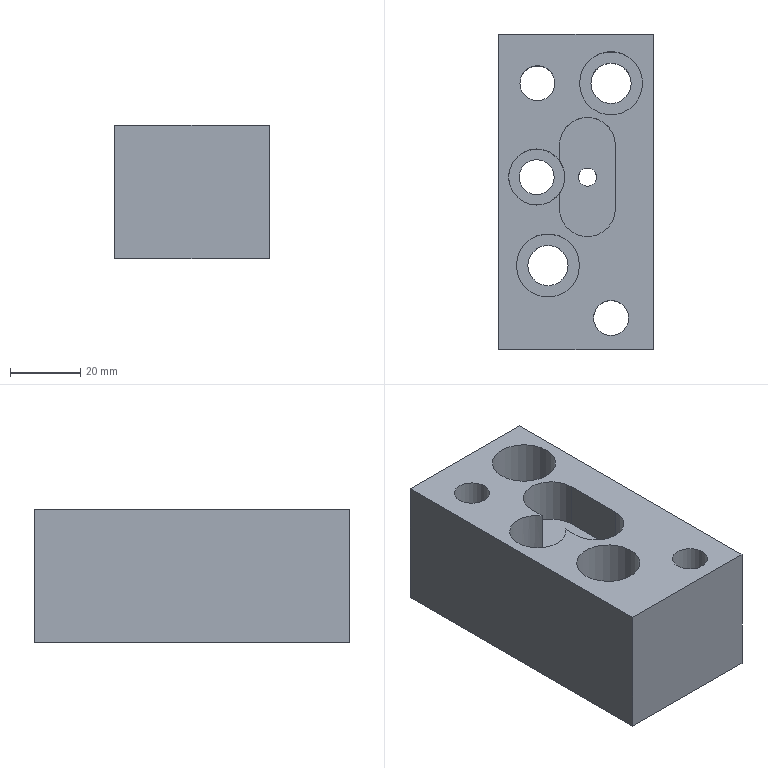Part | STEP file | lll_id142_x_t | 1 solid | 24 faces | box 44 x 90 x 38 mm | volume 119506 mm3 | plane 13 | cylinder 11 | commonest cylinder face diameters 10 x3 16 x3 11.509 x2 18.008 x2 5.206 x1
STEP:
#1=CARTESIAN_POINT('',(784.996,-55.25,0.));
#2=VERTEX_POINT('',#1);
#3=CARTESIAN_POINT('',(794.,-55.25,0.));
#4=DIRECTION('',(0.,0.,-1.));
#5=DIRECTION('',(-1.,0.,0.));
#6=AXIS2_PLACEMENT_3D('',#3,#4,#5);
#7=CIRCLE('',#6,9.004);
#8=EDGE_CURVE('',#2,#2,#7,.T.);
#9=ORIENTED_EDGE('',*,*,#8,.T.);
#10=EDGE_LOOP('',(#9));
#11=FACE_BOUND('',#10,.T.);
#12=CARTESIAN_POINT('',(780.,-79.25,0.));
#13=VERTEX_POINT('',#12);
#14=CARTESIAN_POINT('',(780.,10.75,0.));
#15=VERTEX_POINT('',#14);
#16=CARTESIAN_POINT('',(780.,0.,0.));
#17=DIRECTION('',(0.,1.,0.));
#18=VECTOR('',#17,1.);
#19=LINE('',#16,#18);
#20=EDGE_CURVE('',#13,#15,#19,.T.);
#21=ORIENTED_EDGE('',*,*,#20,.F.);
#22=CARTESIAN_POINT('',(824.,-79.25,0.));
#23=VERTEX_POINT('',#22);
#24=CARTESIAN_POINT('',(829.,-79.25,0.));
#25=DIRECTION('',(-1.,0.,0.));
#26=VECTOR('',#25,1.);
#27=LINE('',#24,#26);
#28=EDGE_CURVE('',#23,#13,#27,.T.);
#29=ORIENTED_EDGE('',*,*,#28,.F.);
#30=CARTESIAN_POINT('',(824.,10.75,0.));
#31=VERTEX_POINT('',#30);
#32=CARTESIAN_POINT('',(824.,0.,0.));
#33=DIRECTION('',(0.,1.,0.));
#34=VECTOR('',#33,1.);
#35=LINE('',#32,#34);
#36=EDGE_CURVE('',#23,#31,#35,.T.);
#37=ORIENTED_EDGE('',*,*,#36,.T.);
#38=CARTESIAN_POINT('',(829.,10.75,0.));
#39=DIRECTION('',(-1.,0.,0.));
#40=VECTOR('',#39,1.);
#41=LINE('',#38,#40);
#42=EDGE_CURVE('',#31,#15,#41,.T.);
#43=ORIENTED_EDGE('',*,*,#42,.T.);
#44=EDGE_LOOP('',(#21,#29,#37,#43));
#45=FACE_BOUND('',#44,.T.);
#46=CARTESIAN_POINT('',(796.,-3.25,0.));
#47=VERTEX_POINT('',#46);
#48=CARTESIAN_POINT('',(791.,-3.25,0.));
#49=DIRECTION('',(0.,0.,1.));
#50=DIRECTION('',(1.,0.,0.));
#51=AXIS2_PLACEMENT_3D('',#48,#49,#50);
#52=CIRCLE('',#51,5.);
#53=EDGE_CURVE('',#47,#47,#52,.T.);
#54=ORIENTED_EDGE('',*,*,#53,.F.);
#55=EDGE_LOOP('',(#54));
#56=FACE_BOUND('',#55,.T.);
#57=CARTESIAN_POINT('',(802.996,-3.25,0.));
#58=VERTEX_POINT('',#57);
#59=CARTESIAN_POINT('',(812.,-3.25,0.));
#60=DIRECTION('',(0.,0.,-1.));
#61=DIRECTION('',(-1.,0.,0.));
#62=AXIS2_PLACEMENT_3D('',#59,#60,#61);
#63=CIRCLE('',#62,9.004);
#64=EDGE_CURVE('',#58,#58,#63,.T.);
#65=ORIENTED_EDGE('',*,*,#64,.T.);
#66=EDGE_LOOP('',(#65));
#67=FACE_BOUND('',#66,.T.);
#68=CARTESIAN_POINT('',(817.,-70.25,0.));
#69=VERTEX_POINT('',#68);
#70=CARTESIAN_POINT('',(812.,-70.25,0.));
#71=DIRECTION('',(0.,0.,1.));
#72=DIRECTION('',(1.,0.,0.));
#73=AXIS2_PLACEMENT_3D('',#70,#71,#72);
#74=CIRCLE('',#73,5.);
#75=EDGE_CURVE('',#69,#69,#74,.T.);
#76=ORIENTED_EDGE('',*,*,#75,.F.);
#77=EDGE_LOOP('',(#76));
#78=FACE_BOUND('',#77,.T.);
#79=CARTESIAN_POINT('',(797.273,-39.,0.));
#80=VERTEX_POINT('',#79);
#81=CARTESIAN_POINT('',(813.273,-39.,0.));
#82=VERTEX_POINT('',#81);
#83=CARTESIAN_POINT('',(805.273,-39.,0.));
#84=DIRECTION('',(0.,0.,1.));
#85=DIRECTION('',(1.,0.,0.));
#86=AXIS2_PLACEMENT_3D('',#83,#84,#85);
#87=CIRCLE('',#86,8.);
#88=EDGE_CURVE('',#80,#82,#87,.T.);
#89=ORIENTED_EDGE('',*,*,#88,.F.);
#90=CARTESIAN_POINT('',(797.273,-34.664,0.));
#91=VERTEX_POINT('',#90);
#92=CARTESIAN_POINT('',(797.273,-79.25,0.));
#93=DIRECTION('',(0.,1.,0.));
#94=VECTOR('',#93,1.);
#95=LINE('',#92,#94);
#96=EDGE_CURVE('',#80,#91,#95,.T.);
#97=ORIENTED_EDGE('',*,*,#96,.T.);
#98=CARTESIAN_POINT('',(797.273,-25.336,0.));
#99=VERTEX_POINT('',#98);
#100=CARTESIAN_POINT('',(790.773,-30.,0.));
#101=DIRECTION('',(0.,0.,1.));
#102=DIRECTION('',(1.,0.,0.));
#103=AXIS2_PLACEMENT_3D('',#100,#101,#102);
#104=CIRCLE('',#103,8.);
#105=EDGE_CURVE('',#99,#91,#104,.T.);
#106=ORIENTED_EDGE('',*,*,#105,.F.);
#107=CARTESIAN_POINT('',(797.273,-21.,0.));
#108=VERTEX_POINT('',#107);
#109=CARTESIAN_POINT('',(797.273,-79.25,0.));
#110=DIRECTION('',(0.,1.,0.));
#111=VECTOR('',#110,1.);
#112=LINE('',#109,#111);
#113=EDGE_CURVE('',#99,#108,#112,.T.);
#114=ORIENTED_EDGE('',*,*,#113,.T.);
#115=CARTESIAN_POINT('',(813.273,-21.,0.));
#116=VERTEX_POINT('',#115);
#117=CARTESIAN_POINT('',(805.273,-21.,0.));
#118=DIRECTION('',(0.,0.,1.));
#119=DIRECTION('',(1.,0.,0.));
#120=AXIS2_PLACEMENT_3D('',#117,#118,#119);
#121=CIRCLE('',#120,8.);
#122=EDGE_CURVE('',#116,#108,#121,.T.);
#123=ORIENTED_EDGE('',*,*,#122,.F.);
#124=CARTESIAN_POINT('',(813.273,-79.25,0.));
#125=DIRECTION('',(0.,1.,0.));
#126=VECTOR('',#125,1.);
#127=LINE('',#124,#126);
#128=EDGE_CURVE('',#82,#116,#127,.T.);
#129=ORIENTED_EDGE('',*,*,#128,.F.);
#130=EDGE_LOOP('',(#89,#97,#106,#114,#123,#129));
#131=FACE_BOUND('',#130,.T.);
#132=CARTESIAN_POINT('',(829.,-79.25,0.));
#133=DIRECTION('',(0.,0.,1.));
#134=DIRECTION('',(1.,0.,0.));
#135=AXIS2_PLACEMENT_3D('',#132,#133,#134);
#136=PLANE('',#135);
#137=ADVANCED_FACE('',(#11,#45,#56,#67,#78,#131),#136,.T.);
#138=CARTESIAN_POINT('',(798.773,-30.,-28.));
#139=VERTEX_POINT('',#138);
#140=CARTESIAN_POINT('',(790.773,-30.,-28.));
#141=DIRECTION('',(0.,0.,-1.));
#142=DIRECTION('',(1.,0.,0.));
#143=AXIS2_PLACEMENT_3D('',#140,#141,#142);
#144=CIRCLE('',#143,8.);
#145=EDGE_CURVE('',#139,#139,#144,.T.);
#146=ORIENTED_EDGE('',*,*,#145,.T.);
#147=EDGE_LOOP('',(#146));
#148=FACE_BOUND('',#147,.T.);
#149=CARTESIAN_POINT('',(797.273,-25.336,-13.));
#150=VERTEX_POINT('',#149);
#151=CARTESIAN_POINT('',(797.273,-25.336,0.));
#152=DIRECTION('',(0.,0.,-1.));
#153=VECTOR('',#152,1.);
#154=LINE('',#151,#153);
#155=EDGE_CURVE('',#99,#150,#154,.T.);
#156=ORIENTED_EDGE('',*,*,#155,.F.);
#157=ORIENTED_EDGE('',*,*,#105,.T.);
#158=CARTESIAN_POINT('',(797.273,-34.664,-13.));
#159=VERTEX_POINT('',#158);
#160=CARTESIAN_POINT('',(797.273,-34.664,-13.));
#161=DIRECTION('',(0.,0.,1.));
#162=VECTOR('',#161,1.);
#163=LINE('',#160,#162);
#164=EDGE_CURVE('',#159,#91,#163,.T.);
#165=ORIENTED_EDGE('',*,*,#164,.F.);
#166=CARTESIAN_POINT('',(790.773,-30.,-13.));
#167=DIRECTION('',(0.,0.,1.));
#168=DIRECTION('',(-1.,0.,0.));
#169=AXIS2_PLACEMENT_3D('',#166,#167,#168);
#170=CIRCLE('',#169,8.);
#171=EDGE_CURVE('',#159,#150,#170,.T.);
#172=ORIENTED_EDGE('',*,*,#171,.T.);
#173=EDGE_LOOP('',(#156,#157,#165,#172));
#174=FACE_BOUND('',#173,.T.);
#175=CARTESIAN_POINT('',(790.773,-30.,-28.));
#176=DIRECTION('',(0.,0.,1.));
#177=DIRECTION('',(1.,0.,0.));
#178=AXIS2_PLACEMENT_3D('',#175,#176,#177);
#179=CYLINDRICAL_SURFACE('',#178,8.);
#180=ADVANCED_FACE('',(#148,#174),#179,.F.);
#181=CARTESIAN_POINT('',(780.,10.75,-38.));
#182=VERTEX_POINT('',#181);
#183=CARTESIAN_POINT('',(780.,10.75,0.));
#184=DIRECTION('',(0.,0.,-1.));
#185=VECTOR('',#184,1.);
#186=LINE('',#183,#185);
#187=EDGE_CURVE('',#15,#182,#186,.T.);
#188=ORIENTED_EDGE('',*,*,#187,.F.);
#189=ORIENTED_EDGE('',*,*,#42,.F.);
#190=CARTESIAN_POINT('',(824.,10.75,-38.));
#191=VERTEX_POINT('',#190);
#192=CARTESIAN_POINT('',(824.,10.75,0.));
#193=DIRECTION('',(0.,0.,-1.));
#194=VECTOR('',#193,1.);
#195=LINE('',#192,#194);
#196=EDGE_CURVE('',#31,#191,#195,.T.);
#197=ORIENTED_EDGE('',*,*,#196,.T.);
#198=CARTESIAN_POINT('',(829.,10.75,-38.));
#199=DIRECTION('',(-1.,0.,0.));
#200=VECTOR('',#199,1.);
#201=LINE('',#198,#200);
#202=EDGE_CURVE('',#191,#182,#201,.T.);
#203=ORIENTED_EDGE('',*,*,#202,.T.);
#204=EDGE_LOOP('',(#188,#189,#197,#203));
#205=FACE_OUTER_BOUND('',#204,.T.);
#206=CARTESIAN_POINT('',(829.,10.75,0.));
#207=DIRECTION('',(0.,1.,0.));
#208=DIRECTION('',(0.,0.,1.));
#209=AXIS2_PLACEMENT_3D('',#206,#207,#208);
#210=PLANE('',#209);
#211=ADVANCED_FACE('',(#205),#210,.T.);
#212=CARTESIAN_POINT('',(802.67,-30.,-38.));
#213=VERTEX_POINT('',#212);
#214=CARTESIAN_POINT('',(805.273,-30.,-38.));
#215=DIRECTION('',(0.,0.,-1.));
#216=DIRECTION('',(-1.,0.,0.));
#217=AXIS2_PLACEMENT_3D('',#214,#215,#216);
#218=CIRCLE('',#217,2.603);
#219=EDGE_CURVE('',#213,#213,#218,.T.);
#220=ORIENTED_EDGE('',*,*,#219,.F.);
#221=EDGE_LOOP('',(#220));
#222=FACE_BOUND('',#221,.T.);
#223=CARTESIAN_POINT('',(785.773,-30.,-38.));
#224=VERTEX_POINT('',#223);
#225=CARTESIAN_POINT('',(790.773,-30.,-38.));
#226=DIRECTION('',(0.,0.,-1.));
#227=DIRECTION('',(-1.,0.,0.));
#228=AXIS2_PLACEMENT_3D('',#225,#226,#227);
#229=CIRCLE('',#228,5.);
#230=EDGE_CURVE('',#224,#224,#229,.T.);
#231=ORIENTED_EDGE('',*,*,#230,.F.);
#232=EDGE_LOOP('',(#231));
#233=FACE_BOUND('',#232,.T.);
#234=CARTESIAN_POINT('',(807.,-70.25,-38.));
#235=VERTEX_POINT('',#234);
#236=CARTESIAN_POINT('',(812.,-70.25,-38.));
#237=DIRECTION('',(0.,0.,-1.));
#238=DIRECTION('',(-1.,0.,0.));
#239=AXIS2_PLACEMENT_3D('',#236,#237,#238);
#240=CIRCLE('',#239,5.);
#241=EDGE_CURVE('',#235,#235,#240,.T.);
#242=ORIENTED_EDGE('',*,*,#241,.F.);
#243=EDGE_LOOP('',(#242));
#244=FACE_BOUND('',#243,.T.);
#245=CARTESIAN_POINT('',(788.245,-55.25,-38.));
#246=VERTEX_POINT('',#245);
#247=CARTESIAN_POINT('',(794.,-55.25,-38.));
#248=DIRECTION('',(0.,0.,-1.));
#249=DIRECTION('',(-1.,0.,0.));
#250=AXIS2_PLACEMENT_3D('',#247,#248,#249);
#251=CIRCLE('',#250,5.755);
#252=EDGE_CURVE('',#246,#246,#251,.T.);
#253=ORIENTED_EDGE('',*,*,#252,.F.);
#254=EDGE_LOOP('',(#253));
#255=FACE_BOUND('',#254,.T.);
#256=CARTESIAN_POINT('',(806.245,-3.25,-38.));
#257=VERTEX_POINT('',#256);
#258=CARTESIAN_POINT('',(812.,-3.25,-38.));
#259=DIRECTION('',(0.,0.,-1.));
#260=DIRECTION('',(-1.,0.,0.));
#261=AXIS2_PLACEMENT_3D('',#258,#259,#260);
#262=CIRCLE('',#261,5.755);
#263=EDGE_CURVE('',#257,#257,#262,.T.);
#264=ORIENTED_EDGE('',*,*,#263,.F.);
#265=EDGE_LOOP('',(#264));
#266=FACE_BOUND('',#265,.T.);
#267=CARTESIAN_POINT('',(786.,-3.25,-38.));
#268=VERTEX_POINT('',#267);
#269=CARTESIAN_POINT('',(791.,-3.25,-38.));
#270=DIRECTION('',(0.,0.,-1.));
#271=DIRECTION('',(-1.,0.,0.));
#272=AXIS2_PLACEMENT_3D('',#269,#270,#271);
#273=CIRCLE('',#272,5.);
#274=EDGE_CURVE('',#268,#268,#273,.T.);
#275=ORIENTED_EDGE('',*,*,#274,.F.);
#276=EDGE_LOOP('',(#275));
#277=FACE_BOUND('',#276,.T.);
#278=CARTESIAN_POINT('',(780.,-79.25,-38.));
#279=VERTEX_POINT('',#278);
#280=CARTESIAN_POINT('',(780.,0.,-38.));
#281=DIRECTION('',(0.,-1.,0.));
#282=VECTOR('',#281,1.);
#283=LINE('',#280,#282);
#284=EDGE_CURVE('',#182,#279,#283,.T.);
#285=ORIENTED_EDGE('',*,*,#284,.F.);
#286=ORIENTED_EDGE('',*,*,#202,.F.);
#287=CARTESIAN_POINT('',(824.,-79.25,-38.));
#288=VERTEX_POINT('',#287);
#289=CARTESIAN_POINT('',(824.,0.,-38.));
#290=DIRECTION('',(0.,-1.,0.));
#291=VECTOR('',#290,1.);
#292=LINE('',#289,#291);
#293=EDGE_CURVE('',#191,#288,#292,.T.);
#294=ORIENTED_EDGE('',*,*,#293,.T.);
#295=CARTESIAN_POINT('',(829.,-79.25,-38.));
#296=DIRECTION('',(-1.,0.,0.));
#297=VECTOR('',#296,1.);
#298=LINE('',#295,#297);
#299=EDGE_CURVE('',#288,#279,#298,.T.);
#300=ORIENTED_EDGE('',*,*,#299,.T.);
#301=EDGE_LOOP('',(#285,#286,#294,#300));
#302=FACE_BOUND('',#301,.T.);
#303=CARTESIAN_POINT('',(829.,-19.25,-38.));
#304=DIRECTION('',(0.,0.,-1.));
#305=DIRECTION('',(-1.,0.,0.));
#306=AXIS2_PLACEMENT_3D('',#303,#304,#305);
#307=PLANE('',#306);
#308=ADVANCED_FACE('',(#222,#233,#244,#255,#266,#277,#302),#307,.T.);
#309=CARTESIAN_POINT('',(780.,-79.25,0.));
#310=DIRECTION('',(0.,0.,1.));
#311=VECTOR('',#310,1.);
#312=LINE('',#309,#311);
#313=EDGE_CURVE('',#279,#13,#312,.T.);
#314=ORIENTED_EDGE('',*,*,#313,.F.);
#315=ORIENTED_EDGE('',*,*,#299,.F.);
#316=CARTESIAN_POINT('',(824.,-79.25,0.));
#317=DIRECTION('',(0.,0.,1.));
#318=VECTOR('',#317,1.);
#319=LINE('',#316,#318);
#320=EDGE_CURVE('',#288,#23,#319,.T.);
#321=ORIENTED_EDGE('',*,*,#320,.T.);
#322=ORIENTED_EDGE('',*,*,#28,.T.);
#323=EDGE_LOOP('',(#314,#315,#321,#322));
#324=FACE_OUTER_BOUND('',#323,.T.);
#325=CARTESIAN_POINT('',(829.,-79.25,-38.));
#326=DIRECTION('',(0.,-1.,0.));
#327=DIRECTION('',(0.,0.,-1.));
#328=AXIS2_PLACEMENT_3D('',#325,#326,#327);
#329=PLANE('',#328);
#330=ADVANCED_FACE('',(#324),#329,.T.);
#331=ORIENTED_EDGE('',*,*,#196,.F.);
#332=ORIENTED_EDGE('',*,*,#36,.F.);
#333=ORIENTED_EDGE('',*,*,#320,.F.);
#334=ORIENTED_EDGE('',*,*,#293,.F.);
#335=EDGE_LOOP('',(#331,#332,#333,#334));
#336=FACE_OUTER_BOUND('',#335,.T.);
#337=CARTESIAN_POINT('',(824.,0.,0.));
#338=DIRECTION('',(-1.,0.,0.));
#339=DIRECTION('',(0.,0.,1.));
#340=AXIS2_PLACEMENT_3D('',#337,#338,#339);
#341=PLANE('',#340);
#342=ADVANCED_FACE('',(#336),#341,.F.);
#343=ORIENTED_EDGE('',*,*,#187,.T.);
#344=ORIENTED_EDGE('',*,*,#284,.T.);
#345=ORIENTED_EDGE('',*,*,#313,.T.);
#346=ORIENTED_EDGE('',*,*,#20,.T.);
#347=EDGE_LOOP('',(#343,#344,#345,#346));
#348=FACE_OUTER_BOUND('',#347,.T.);
#349=CARTESIAN_POINT('',(780.,0.,0.));
#350=DIRECTION('',(-1.,0.,0.));
#351=DIRECTION('',(0.,0.,1.));
#352=AXIS2_PLACEMENT_3D('',#349,#350,#351);
#353=PLANE('',#352);
#354=ADVANCED_FACE('',(#348),#353,.T.);
#355=ORIENTED_EDGE('',*,*,#274,.T.);
#356=EDGE_LOOP('',(#355));
#357=FACE_BOUND('',#356,.T.);
#358=ORIENTED_EDGE('',*,*,#53,.T.);
#359=EDGE_LOOP('',(#358));
#360=FACE_BOUND('',#359,.T.);
#361=CARTESIAN_POINT('',(791.,-3.25,2.));
#362=DIRECTION('',(0.,0.,-1.));
#363=DIRECTION('',(-1.,0.,0.));
#364=AXIS2_PLACEMENT_3D('',#361,#362,#363);
#365=CYLINDRICAL_SURFACE('',#364,5.);
#366=ADVANCED_FACE('',(#357,#360),#365,.F.);
#367=ORIENTED_EDGE('',*,*,#263,.T.);
#368=EDGE_LOOP('',(#367));
#369=FACE_BOUND('',#368,.T.);
#370=CARTESIAN_POINT('',(806.245,-3.25,-13.));
#371=VERTEX_POINT('',#370);
#372=CARTESIAN_POINT('',(812.,-3.25,-13.));
#373=DIRECTION('',(0.,0.,-1.));
#374=DIRECTION('',(-1.,0.,0.));
#375=AXIS2_PLACEMENT_3D('',#372,#373,#374);
#376=CIRCLE('',#375,5.755);
#377=EDGE_CURVE('',#371,#371,#376,.T.);
#378=ORIENTED_EDGE('',*,*,#377,.F.);
#379=EDGE_LOOP('',(#378));
#380=FACE_BOUND('',#379,.T.);
#381=CARTESIAN_POINT('',(812.,-3.25,2.));
#382=DIRECTION('',(0.,0.,-1.));
#383=DIRECTION('',(-1.,0.,0.));
#384=AXIS2_PLACEMENT_3D('',#381,#382,#383);
#385=CYLINDRICAL_SURFACE('',#384,5.755);
#386=ADVANCED_FACE('',(#369,#380),#385,.F.);
#387=ORIENTED_EDGE('',*,*,#377,.T.);
#388=EDGE_LOOP('',(#387));
#389=FACE_BOUND('',#388,.T.);
#390=CARTESIAN_POINT('',(802.996,-3.25,-13.));
#391=VERTEX_POINT('',#390);
#392=CARTESIAN_POINT('',(812.,-3.25,-13.));
#393=DIRECTION('',(0.,0.,-1.));
#394=DIRECTION('',(-1.,0.,0.));
#395=AXIS2_PLACEMENT_3D('',#392,#393,#394);
#396=CIRCLE('',#395,9.004);
#397=EDGE_CURVE('',#391,#391,#396,.T.);
#398=ORIENTED_EDGE('',*,*,#397,.F.);
#399=EDGE_LOOP('',(#398));
#400=FACE_BOUND('',#399,.T.);
#401=CARTESIAN_POINT('',(812.,-3.25,-13.));
#402=DIRECTION('',(0.,0.,-1.));
#403=DIRECTION('',(-1.,0.,0.));
#404=AXIS2_PLACEMENT_3D('',#401,#402,#403);
#405=PLANE('',#404);
#406=ADVANCED_FACE('',(#389,#400),#405,.F.);
#407=ORIENTED_EDGE('',*,*,#397,.T.);
#408=EDGE_LOOP('',(#407));
#409=FACE_BOUND('',#408,.T.);
#410=ORIENTED_EDGE('',*,*,#64,.F.);
#411=EDGE_LOOP('',(#410));
#412=FACE_BOUND('',#411,.T.);
#413=CARTESIAN_POINT('',(812.,-3.25,0.));
#414=DIRECTION('',(0.,0.,-1.));
#415=DIRECTION('',(-1.,0.,0.));
#416=AXIS2_PLACEMENT_3D('',#413,#414,#415);
#417=CYLINDRICAL_SURFACE('',#416,9.004);
#418=ADVANCED_FACE('',(#409,#412),#417,.F.);
#419=ORIENTED_EDGE('',*,*,#252,.T.);
#420=EDGE_LOOP('',(#419));
#421=FACE_BOUND('',#420,.T.);
#422=CARTESIAN_POINT('',(788.245,-55.25,-13.));
#423=VERTEX_POINT('',#422);
#424=CARTESIAN_POINT('',(794.,-55.25,-13.));
#425=DIRECTION('',(0.,0.,-1.));
#426=DIRECTION('',(-1.,0.,0.));
#427=AXIS2_PLACEMENT_3D('',#424,#425,#426);
#428=CIRCLE('',#427,5.755);
#429=EDGE_CURVE('',#423,#423,#428,.T.);
#430=ORIENTED_EDGE('',*,*,#429,.F.);
#431=EDGE_LOOP('',(#430));
#432=FACE_BOUND('',#431,.T.);
#433=CARTESIAN_POINT('',(794.,-55.25,2.));
#434=DIRECTION('',(0.,0.,-1.));
#435=DIRECTION('',(-1.,0.,0.));
#436=AXIS2_PLACEMENT_3D('',#433,#434,#435);
#437=CYLINDRICAL_SURFACE('',#436,5.755);
#438=ADVANCED_FACE('',(#421,#432),#437,.F.);
#439=ORIENTED_EDGE('',*,*,#429,.T.);
#440=EDGE_LOOP('',(#439));
#441=FACE_BOUND('',#440,.T.);
#442=CARTESIAN_POINT('',(784.996,-55.25,-13.));
#443=VERTEX_POINT('',#442);
#444=CARTESIAN_POINT('',(794.,-55.25,-13.));
#445=DIRECTION('',(0.,0.,-1.));
#446=DIRECTION('',(-1.,0.,0.));
#447=AXIS2_PLACEMENT_3D('',#444,#445,#446);
#448=CIRCLE('',#447,9.004);
#449=EDGE_CURVE('',#443,#443,#448,.T.);
#450=ORIENTED_EDGE('',*,*,#449,.F.);
#451=EDGE_LOOP('',(#450));
#452=FACE_BOUND('',#451,.T.);
#453=CARTESIAN_POINT('',(794.,-55.25,-13.));
#454=DIRECTION('',(0.,0.,-1.));
#455=DIRECTION('',(-1.,0.,0.));
#456=AXIS2_PLACEMENT_3D('',#453,#454,#455);
#457=PLANE('',#456);
#458=ADVANCED_FACE('',(#441,#452),#457,.F.);
#459=ORIENTED_EDGE('',*,*,#449,.T.);
#460=EDGE_LOOP('',(#459));
#461=FACE_BOUND('',#460,.T.);
#462=ORIENTED_EDGE('',*,*,#8,.F.);
#463=EDGE_LOOP('',(#462));
#464=FACE_BOUND('',#463,.T.);
#465=CARTESIAN_POINT('',(794.,-55.25,0.));
#466=DIRECTION('',(0.,0.,-1.));
#467=DIRECTION('',(-1.,0.,0.));
#468=AXIS2_PLACEMENT_3D('',#465,#466,#467);
#469=CYLINDRICAL_SURFACE('',#468,9.004);
#470=ADVANCED_FACE('',(#461,#464),#469,.F.);
#471=ORIENTED_EDGE('',*,*,#75,.T.);
#472=EDGE_LOOP('',(#471));
#473=FACE_BOUND('',#472,.T.);
#474=ORIENTED_EDGE('',*,*,#241,.T.);
#475=EDGE_LOOP('',(#474));
#476=FACE_BOUND('',#475,.T.);
#477=CARTESIAN_POINT('',(812.,-70.25,2.));
#478=DIRECTION('',(0.,0.,-1.));
#479=DIRECTION('',(-1.,0.,0.));
#480=AXIS2_PLACEMENT_3D('',#477,#478,#479);
#481=CYLINDRICAL_SURFACE('',#480,5.);
#482=ADVANCED_FACE('',(#473,#476),#481,.F.);
#483=CARTESIAN_POINT('',(785.773,-30.,-28.));
#484=VERTEX_POINT('',#483);
#485=CARTESIAN_POINT('',(790.773,-30.,-28.));
#486=DIRECTION('',(0.,0.,-1.));
#487=DIRECTION('',(-1.,0.,0.));
#488=AXIS2_PLACEMENT_3D('',#485,#486,#487);
#489=CIRCLE('',#488,5.);
#490=EDGE_CURVE('',#484,#484,#489,.T.);
#491=ORIENTED_EDGE('',*,*,#490,.T.);
#492=EDGE_LOOP('',(#491));
#493=FACE_BOUND('',#492,.T.);
#494=ORIENTED_EDGE('',*,*,#145,.F.);
#495=EDGE_LOOP('',(#494));
#496=FACE_BOUND('',#495,.T.);
#497=CARTESIAN_POINT('',(790.773,-30.,-28.));
#498=DIRECTION('',(0.,0.,-1.));
#499=DIRECTION('',(-1.,0.,0.));
#500=AXIS2_PLACEMENT_3D('',#497,#498,#499);
#501=PLANE('',#500);
#502=ADVANCED_FACE('',(#493,#496),#501,.F.);
#503=ORIENTED_EDGE('',*,*,#230,.T.);
#504=EDGE_LOOP('',(#503));
#505=FACE_BOUND('',#504,.T.);
#506=ORIENTED_EDGE('',*,*,#490,.F.);
#507=EDGE_LOOP('',(#506));
#508=FACE_BOUND('',#507,.T.);
#509=CARTESIAN_POINT('',(790.773,-30.,-28.));
#510=DIRECTION('',(0.,0.,-1.));
#511=DIRECTION('',(-1.,0.,0.));
#512=AXIS2_PLACEMENT_3D('',#509,#510,#511);
#513=CYLINDRICAL_SURFACE('',#512,5.);
#514=ADVANCED_FACE('',(#505,#508),#513,.F.);
#515=ORIENTED_EDGE('',*,*,#155,.T.);
#516=CARTESIAN_POINT('',(797.273,-21.,-13.));
#517=VERTEX_POINT('',#516);
#518=CARTESIAN_POINT('',(797.273,-21.,-13.));
#519=DIRECTION('',(0.,1.,0.));
#520=VECTOR('',#519,1.);
#521=LINE('',#518,#520);
#522=EDGE_CURVE('',#150,#517,#521,.T.);
#523=ORIENTED_EDGE('',*,*,#522,.T.);
#524=CARTESIAN_POINT('',(797.273,-21.,7.));
#525=DIRECTION('',(0.,0.,1.));
#526=VECTOR('',#525,1.);
#527=LINE('',#524,#526);
#528=EDGE_CURVE('',#517,#108,#527,.T.);
#529=ORIENTED_EDGE('',*,*,#528,.T.);
#530=ORIENTED_EDGE('',*,*,#113,.F.);
#531=EDGE_LOOP('',(#515,#523,#529,#530));
#532=FACE_OUTER_BOUND('',#531,.T.);
#533=CARTESIAN_POINT('',(797.273,-36.764,7.));
#534=DIRECTION('',(1.,0.,0.));
#535=DIRECTION('',(0.,0.,-1.));
#536=AXIS2_PLACEMENT_3D('',#533,#534,#535);
#537=PLANE('',#536);
#538=ADVANCED_FACE('',(#532),#537,.T.);
#539=CARTESIAN_POINT('',(802.67,-30.,-13.));
#540=VERTEX_POINT('',#539);
#541=CARTESIAN_POINT('',(805.273,-30.,-13.));
#542=DIRECTION('',(0.,0.,-1.));
#543=DIRECTION('',(-1.,0.,0.));
#544=AXIS2_PLACEMENT_3D('',#541,#542,#543);
#545=CIRCLE('',#544,2.603);
#546=EDGE_CURVE('',#540,#540,#545,.T.);
#547=ORIENTED_EDGE('',*,*,#546,.T.);
#548=EDGE_LOOP('',(#547));
#549=FACE_BOUND('',#548,.T.);
#550=CARTESIAN_POINT('',(797.273,-39.,-13.));
#551=VERTEX_POINT('',#550);
#552=CARTESIAN_POINT('',(797.273,-21.,-13.));
#553=DIRECTION('',(0.,1.,0.));
#554=VECTOR('',#553,1.);
#555=LINE('',#552,#554);
#556=EDGE_CURVE('',#551,#159,#555,.T.);
#557=ORIENTED_EDGE('',*,*,#556,.F.);
#558=CARTESIAN_POINT('',(813.273,-39.,-13.));
#559=VERTEX_POINT('',#558);
#560=CARTESIAN_POINT('',(805.273,-39.,-13.));
#561=DIRECTION('',(0.,0.,1.));
#562=DIRECTION('',(0.,1.,0.));
#563=AXIS2_PLACEMENT_3D('',#560,#561,#562);
#564=CIRCLE('',#563,8.);
#565=EDGE_CURVE('',#551,#559,#564,.T.);
#566=ORIENTED_EDGE('',*,*,#565,.T.);
#567=CARTESIAN_POINT('',(813.273,-21.,-13.));
#568=VERTEX_POINT('',#567);
#569=CARTESIAN_POINT('',(813.273,-21.,-13.));
#570=DIRECTION('',(0.,1.,0.));
#571=VECTOR('',#570,1.);
#572=LINE('',#569,#571);
#573=EDGE_CURVE('',#559,#568,#572,.T.);
#574=ORIENTED_EDGE('',*,*,#573,.T.);
#575=CARTESIAN_POINT('',(805.273,-21.,-13.));
#576=DIRECTION('',(0.,0.,1.));
#577=DIRECTION('',(0.,1.,0.));
#578=AXIS2_PLACEMENT_3D('',#575,#576,#577);
#579=CIRCLE('',#578,8.);
#580=EDGE_CURVE('',#568,#517,#579,.T.);
#581=ORIENTED_EDGE('',*,*,#580,.T.);
#582=ORIENTED_EDGE('',*,*,#522,.F.);
#583=ORIENTED_EDGE('',*,*,#171,.F.);
#584=EDGE_LOOP('',(#557,#566,#574,#581,#582,#583));
#585=FACE_BOUND('',#584,.T.);
#586=CARTESIAN_POINT('',(805.773,-39.,-13.));
#587=DIRECTION('',(0.,0.,-1.));
#588=DIRECTION('',(0.,-1.,0.));
#589=AXIS2_PLACEMENT_3D('',#586,#587,#588);
#590=PLANE('',#589);
#591=ADVANCED_FACE('',(#549,#585),#590,.F.);
#592=CARTESIAN_POINT('',(797.273,-39.,7.));
#593=DIRECTION('',(0.,0.,1.));
#594=VECTOR('',#593,1.);
#595=LINE('',#592,#594);
#596=EDGE_CURVE('',#551,#80,#595,.T.);
#597=ORIENTED_EDGE('',*,*,#596,.F.);
#598=ORIENTED_EDGE('',*,*,#556,.T.);
#599=ORIENTED_EDGE('',*,*,#164,.T.);
#600=ORIENTED_EDGE('',*,*,#96,.F.);
#601=EDGE_LOOP('',(#597,#598,#599,#600));
#602=FACE_OUTER_BOUND('',#601,.T.);
#603=CARTESIAN_POINT('',(797.273,-36.764,7.));
#604=DIRECTION('',(1.,0.,0.));
#605=DIRECTION('',(0.,0.,-1.));
#606=AXIS2_PLACEMENT_3D('',#603,#604,#605);
#607=PLANE('',#606);
#608=ADVANCED_FACE('',(#602),#607,.T.);
#609=ORIENTED_EDGE('',*,*,#88,.T.);
#610=CARTESIAN_POINT('',(813.273,-39.,7.));
#611=DIRECTION('',(0.,0.,1.));
#612=VECTOR('',#611,1.);
#613=LINE('',#610,#612);
#614=EDGE_CURVE('',#559,#82,#613,.T.);
#615=ORIENTED_EDGE('',*,*,#614,.F.);
#616=ORIENTED_EDGE('',*,*,#565,.F.);
#617=ORIENTED_EDGE('',*,*,#596,.T.);
#618=EDGE_LOOP('',(#609,#615,#616,#617));
#619=FACE_OUTER_BOUND('',#618,.T.);
#620=CARTESIAN_POINT('',(805.273,-39.,7.));
#621=DIRECTION('',(0.,0.,-1.));
#622=DIRECTION('',(0.,-1.,0.));
#623=AXIS2_PLACEMENT_3D('',#620,#621,#622);
#624=CYLINDRICAL_SURFACE('',#623,8.);
#625=ADVANCED_FACE('',(#619),#624,.F.);
#626=ORIENTED_EDGE('',*,*,#128,.T.);
#627=CARTESIAN_POINT('',(813.273,-21.,7.));
#628=DIRECTION('',(0.,0.,1.));
#629=VECTOR('',#628,1.);
#630=LINE('',#627,#629);
#631=EDGE_CURVE('',#568,#116,#630,.T.);
#632=ORIENTED_EDGE('',*,*,#631,.F.);
#633=ORIENTED_EDGE('',*,*,#573,.F.);
#634=ORIENTED_EDGE('',*,*,#614,.T.);
#635=EDGE_LOOP('',(#626,#632,#633,#634));
#636=FACE_OUTER_BOUND('',#635,.T.);
#637=CARTESIAN_POINT('',(813.273,-21.,7.));
#638=DIRECTION('',(1.,0.,0.));
#639=DIRECTION('',(0.,0.,-1.));
#640=AXIS2_PLACEMENT_3D('',#637,#638,#639);
#641=PLANE('',#640);
#642=ADVANCED_FACE('',(#636),#641,.F.);
#643=ORIENTED_EDGE('',*,*,#122,.T.);
#644=ORIENTED_EDGE('',*,*,#528,.F.);
#645=ORIENTED_EDGE('',*,*,#580,.F.);
#646=ORIENTED_EDGE('',*,*,#631,.T.);
#647=EDGE_LOOP('',(#643,#644,#645,#646));
#648=FACE_OUTER_BOUND('',#647,.T.);
#649=CARTESIAN_POINT('',(805.273,-21.,7.));
#650=DIRECTION('',(0.,0.,-1.));
#651=DIRECTION('',(0.,-1.,0.));
#652=AXIS2_PLACEMENT_3D('',#649,#650,#651);
#653=CYLINDRICAL_SURFACE('',#652,8.);
#654=ADVANCED_FACE('',(#648),#653,.F.);
#655=ORIENTED_EDGE('',*,*,#219,.T.);
#656=EDGE_LOOP('',(#655));
#657=FACE_BOUND('',#656,.T.);
#658=ORIENTED_EDGE('',*,*,#546,.F.);
#659=EDGE_LOOP('',(#658));
#660=FACE_BOUND('',#659,.T.);
#661=CARTESIAN_POINT('',(805.273,-30.,-13.));
#662=DIRECTION('',(0.,0.,-1.));
#663=DIRECTION('',(-1.,0.,0.));
#664=AXIS2_PLACEMENT_3D('',#661,#662,#663);
#665=CYLINDRICAL_SURFACE('',#664,2.603);
#666=ADVANCED_FACE('',(#657,#660),#665,.F.);
#667=CLOSED_SHELL('',(#137,#180,#211,#308,#330,#342,#354,#366,#386,#406,#418,#438,#458,#470,#482,#502,#514,#538,#591,#608,#625,#642,#654,#666));
#668=MANIFOLD_SOLID_BREP('',#667);
#669=(LENGTH_UNIT()NAMED_UNIT(*)SI_UNIT(.MILLI.,.METRE.));
#670=UNCERTAINTY_MEASURE_WITH_UNIT(LENGTH_MEASURE(0.00002),#669,'','');
#671=(NAMED_UNIT(*)PLANE_ANGLE_UNIT()SI_UNIT($,.RADIAN.));
#672=PLANE_ANGLE_MEASURE_WITH_UNIT(PLANE_ANGLE_MEASURE(0.01745),#671);
#673=DIMENSIONAL_EXPONENTS(0.,0.,0.,0.,0.,0.,0.);
#674=(CONVERSION_BASED_UNIT('DEGREE',#672)NAMED_UNIT(#673)PLANE_ANGLE_UNIT());
#675=(NAMED_UNIT(*)SI_UNIT($,.STERADIAN.)SOLID_ANGLE_UNIT());
#676=(GEOMETRIC_REPRESENTATION_CONTEXT(3)GLOBAL_UNCERTAINTY_ASSIGNED_CONTEXT((#670))GLOBAL_UNIT_ASSIGNED_CONTEXT((#669,#674,#675))REPRESENTATION_CONTEXT('',''));
#677=ADVANCED_BREP_SHAPE_REPRESENTATION('',(#668),#676);